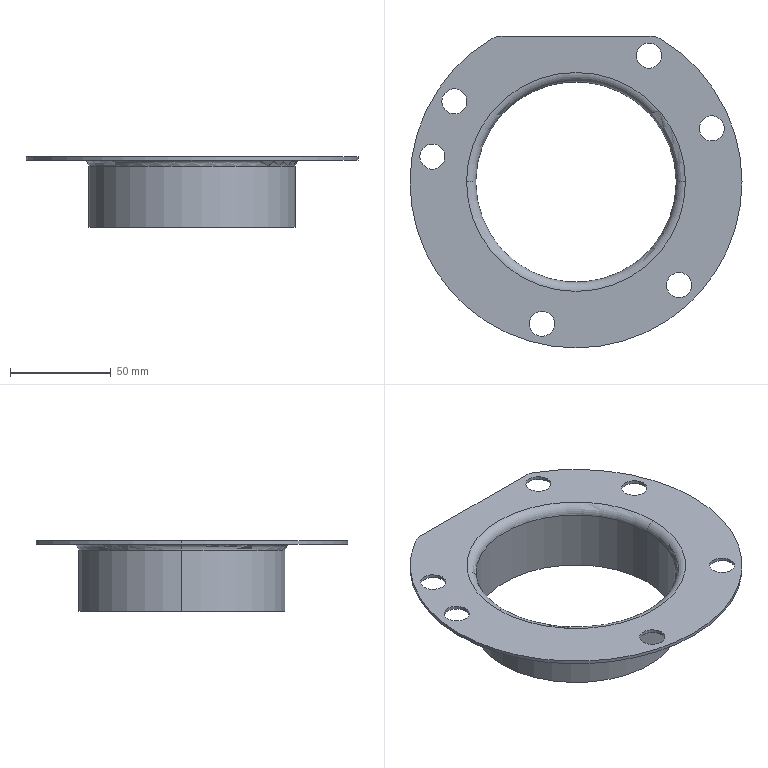Part | SolidWorks | features ICE 2, CirPattern 1, Fillet 1, RevolutionThin 1 | 1 solid | 29 faces | box 165 x 155 x 35 mm | volume 35887 mm3 | cylinder 21 | torus 4 | plane 4 | commonest cylinder face diameters 12.5 x12 165 x3 20 x2 99.6 x2 102.8 x2
STEP:
#1=CARTESIAN_POINT('',(30.,62.787,33.4));
#2=VERTEX_POINT('',#1);
#3=CARTESIAN_POINT('',(42.5,62.787,33.4));
#4=VERTEX_POINT('',#3);
#5=CARTESIAN_POINT('',(36.25,62.787,33.4));
#6=DIRECTION('',(0.,0.,1.));
#7=DIRECTION('',(-1.,0.,0.));
#8=AXIS2_PLACEMENT_3D('',#5,#6,#7);
#9=CIRCLE('',#8,6.25);
#10=EDGE_CURVE('',#2,#4,#9,.T.);
#11=ORIENTED_EDGE('',*,*,#10,.F.);
#12=CARTESIAN_POINT('',(30.,62.787,35.));
#13=VERTEX_POINT('',#12);
#14=CARTESIAN_POINT('',(30.,62.787,-0.001));
#15=DIRECTION('',(0.,0.,1.));
#16=VECTOR('',#15,1000.);
#17=LINE('',#14,#16);
#18=EDGE_CURVE('',#2,#13,#17,.T.);
#19=ORIENTED_EDGE('',*,*,#18,.T.);
#20=CARTESIAN_POINT('',(42.5,62.787,35.));
#21=VERTEX_POINT('',#20);
#22=CARTESIAN_POINT('',(36.25,62.787,35.));
#23=DIRECTION('',(0.,0.,1.));
#24=DIRECTION('',(1.,0.,0.));
#25=AXIS2_PLACEMENT_3D('',#22,#23,#24);
#26=CIRCLE('',#25,6.25);
#27=EDGE_CURVE('',#13,#21,#26,.T.);
#28=ORIENTED_EDGE('',*,*,#27,.T.);
#29=CARTESIAN_POINT('',(42.5,62.787,-0.001));
#30=DIRECTION('',(0.,0.,1.));
#31=VECTOR('',#30,1000.);
#32=LINE('',#29,#31);
#33=EDGE_CURVE('',#4,#21,#32,.T.);
#34=ORIENTED_EDGE('',*,*,#33,.F.);
#35=EDGE_LOOP('',(#11,#19,#28,#34));
#36=FACE_OUTER_BOUND('',#35,.T.);
#37=CARTESIAN_POINT('',(36.25,62.787,-0.001));
#38=DIRECTION('',(0.,0.,1.));
#39=DIRECTION('',(1.,0.,0.));
#40=AXIS2_PLACEMENT_3D('',#37,#38,#39);
#41=CYLINDRICAL_SURFACE('',#40,6.25);
#42=ADVANCED_FACE('',(#36),#41,.F.);
#43=CARTESIAN_POINT('',(61.205,26.571,33.4));
#44=VERTEX_POINT('',#43);
#45=CARTESIAN_POINT('',(73.705,26.571,33.4));
#46=VERTEX_POINT('',#45);
#47=CARTESIAN_POINT('',(67.455,26.571,33.4));
#48=DIRECTION('',(0.,0.,1.));
#49=DIRECTION('',(-1.,0.,0.));
#50=AXIS2_PLACEMENT_3D('',#47,#48,#49);
#51=CIRCLE('',#50,6.25);
#52=EDGE_CURVE('',#44,#46,#51,.T.);
#53=ORIENTED_EDGE('',*,*,#52,.F.);
#54=CARTESIAN_POINT('',(61.205,26.571,35.));
#55=VERTEX_POINT('',#54);
#56=CARTESIAN_POINT('',(61.205,26.571,-0.001));
#57=DIRECTION('',(0.,0.,1.));
#58=VECTOR('',#57,1000.);
#59=LINE('',#56,#58);
#60=EDGE_CURVE('',#44,#55,#59,.T.);
#61=ORIENTED_EDGE('',*,*,#60,.T.);
#62=CARTESIAN_POINT('',(73.705,26.571,35.));
#63=VERTEX_POINT('',#62);
#64=CARTESIAN_POINT('',(67.455,26.571,35.));
#65=DIRECTION('',(0.,0.,1.));
#66=DIRECTION('',(1.,0.,0.));
#67=AXIS2_PLACEMENT_3D('',#64,#65,#66);
#68=CIRCLE('',#67,6.25);
#69=EDGE_CURVE('',#55,#63,#68,.T.);
#70=ORIENTED_EDGE('',*,*,#69,.T.);
#71=CARTESIAN_POINT('',(73.705,26.571,-0.001));
#72=DIRECTION('',(0.,0.,1.));
#73=VECTOR('',#72,1000.);
#74=LINE('',#71,#73);
#75=EDGE_CURVE('',#46,#63,#74,.T.);
#76=ORIENTED_EDGE('',*,*,#75,.F.);
#77=EDGE_LOOP('',(#53,#61,#70,#76));
#78=FACE_OUTER_BOUND('',#77,.T.);
#79=CARTESIAN_POINT('',(67.455,26.571,-0.001));
#80=DIRECTION('',(0.,0.,1.));
#81=DIRECTION('',(1.,0.,0.));
#82=AXIS2_PLACEMENT_3D('',#79,#80,#81);
#83=CYLINDRICAL_SURFACE('',#82,6.25);
#84=ADVANCED_FACE('',(#78),#83,.F.);
#85=CARTESIAN_POINT('',(45.015,-51.265,33.4));
#86=VERTEX_POINT('',#85);
#87=CARTESIAN_POINT('',(57.515,-51.265,33.4));
#88=VERTEX_POINT('',#87);
#89=CARTESIAN_POINT('',(51.265,-51.265,33.4));
#90=DIRECTION('',(0.,0.,1.));
#91=DIRECTION('',(-1.,0.,0.));
#92=AXIS2_PLACEMENT_3D('',#89,#90,#91);
#93=CIRCLE('',#92,6.25);
#94=EDGE_CURVE('',#86,#88,#93,.T.);
#95=ORIENTED_EDGE('',*,*,#94,.F.);
#96=CARTESIAN_POINT('',(45.015,-51.265,35.));
#97=VERTEX_POINT('',#96);
#98=CARTESIAN_POINT('',(45.015,-51.265,-0.001));
#99=DIRECTION('',(0.,0.,1.));
#100=VECTOR('',#99,1000.);
#101=LINE('',#98,#100);
#102=EDGE_CURVE('',#86,#97,#101,.T.);
#103=ORIENTED_EDGE('',*,*,#102,.T.);
#104=CARTESIAN_POINT('',(57.515,-51.265,35.));
#105=VERTEX_POINT('',#104);
#106=CARTESIAN_POINT('',(51.265,-51.265,35.));
#107=DIRECTION('',(0.,0.,1.));
#108=DIRECTION('',(1.,0.,0.));
#109=AXIS2_PLACEMENT_3D('',#106,#107,#108);
#110=CIRCLE('',#109,6.25);
#111=EDGE_CURVE('',#97,#105,#110,.T.);
#112=ORIENTED_EDGE('',*,*,#111,.T.);
#113=CARTESIAN_POINT('',(57.515,-51.265,-0.001));
#114=DIRECTION('',(0.,0.,1.));
#115=VECTOR('',#114,1000.);
#116=LINE('',#113,#115);
#117=EDGE_CURVE('',#88,#105,#116,.T.);
#118=ORIENTED_EDGE('',*,*,#117,.F.);
#119=EDGE_LOOP('',(#95,#103,#112,#118));
#120=FACE_OUTER_BOUND('',#119,.T.);
#121=CARTESIAN_POINT('',(51.265,-51.265,-0.001));
#122=DIRECTION('',(0.,0.,1.));
#123=DIRECTION('',(1.,0.,0.));
#124=AXIS2_PLACEMENT_3D('',#121,#122,#123);
#125=CYLINDRICAL_SURFACE('',#124,6.25);
#126=ADVANCED_FACE('',(#120),#125,.F.);
#127=CARTESIAN_POINT('',(-23.175,-70.497,33.4));
#128=VERTEX_POINT('',#127);
#129=CARTESIAN_POINT('',(-10.675,-70.497,33.4));
#130=VERTEX_POINT('',#129);
#131=CARTESIAN_POINT('',(-16.925,-70.497,33.4));
#132=DIRECTION('',(0.,0.,1.));
#133=DIRECTION('',(-1.,0.,0.));
#134=AXIS2_PLACEMENT_3D('',#131,#132,#133);
#135=CIRCLE('',#134,6.25);
#136=EDGE_CURVE('',#128,#130,#135,.T.);
#137=ORIENTED_EDGE('',*,*,#136,.F.);
#138=CARTESIAN_POINT('',(-23.175,-70.497,35.));
#139=VERTEX_POINT('',#138);
#140=CARTESIAN_POINT('',(-23.175,-70.497,-0.001));
#141=DIRECTION('',(0.,0.,1.));
#142=VECTOR('',#141,1000.);
#143=LINE('',#140,#142);
#144=EDGE_CURVE('',#128,#139,#143,.T.);
#145=ORIENTED_EDGE('',*,*,#144,.T.);
#146=CARTESIAN_POINT('',(-10.675,-70.497,35.));
#147=VERTEX_POINT('',#146);
#148=CARTESIAN_POINT('',(-16.925,-70.497,35.));
#149=DIRECTION('',(0.,0.,1.));
#150=DIRECTION('',(1.,0.,0.));
#151=AXIS2_PLACEMENT_3D('',#148,#149,#150);
#152=CIRCLE('',#151,6.25);
#153=EDGE_CURVE('',#139,#147,#152,.T.);
#154=ORIENTED_EDGE('',*,*,#153,.T.);
#155=CARTESIAN_POINT('',(-10.675,-70.497,-0.001));
#156=DIRECTION('',(0.,0.,1.));
#157=VECTOR('',#156,1000.);
#158=LINE('',#155,#157);
#159=EDGE_CURVE('',#130,#147,#158,.T.);
#160=ORIENTED_EDGE('',*,*,#159,.F.);
#161=EDGE_LOOP('',(#137,#145,#154,#160));
#162=FACE_OUTER_BOUND('',#161,.T.);
#163=CARTESIAN_POINT('',(-16.925,-70.497,-0.001));
#164=DIRECTION('',(0.,0.,1.));
#165=DIRECTION('',(1.,0.,0.));
#166=AXIS2_PLACEMENT_3D('',#163,#164,#165);
#167=CYLINDRICAL_SURFACE('',#166,6.25);
#168=ADVANCED_FACE('',(#162),#167,.F.);
#169=CARTESIAN_POINT('',(-77.649,12.589,33.4));
#170=VERTEX_POINT('',#169);
#171=CARTESIAN_POINT('',(-65.149,12.589,33.4));
#172=VERTEX_POINT('',#171);
#173=CARTESIAN_POINT('',(-71.399,12.589,33.4));
#174=DIRECTION('',(0.,0.,1.));
#175=DIRECTION('',(-1.,0.,0.));
#176=AXIS2_PLACEMENT_3D('',#173,#174,#175);
#177=CIRCLE('',#176,6.25);
#178=EDGE_CURVE('',#170,#172,#177,.T.);
#179=ORIENTED_EDGE('',*,*,#178,.F.);
#180=CARTESIAN_POINT('',(-77.649,12.589,35.));
#181=VERTEX_POINT('',#180);
#182=CARTESIAN_POINT('',(-77.649,12.589,-0.001));
#183=DIRECTION('',(0.,0.,1.));
#184=VECTOR('',#183,1000.);
#185=LINE('',#182,#184);
#186=EDGE_CURVE('',#170,#181,#185,.T.);
#187=ORIENTED_EDGE('',*,*,#186,.T.);
#188=CARTESIAN_POINT('',(-65.149,12.589,35.));
#189=VERTEX_POINT('',#188);
#190=CARTESIAN_POINT('',(-71.399,12.589,35.));
#191=DIRECTION('',(0.,0.,1.));
#192=DIRECTION('',(1.,0.,0.));
#193=AXIS2_PLACEMENT_3D('',#190,#191,#192);
#194=CIRCLE('',#193,6.25);
#195=EDGE_CURVE('',#181,#189,#194,.T.);
#196=ORIENTED_EDGE('',*,*,#195,.T.);
#197=CARTESIAN_POINT('',(-65.149,12.589,-0.001));
#198=DIRECTION('',(0.,0.,1.));
#199=VECTOR('',#198,1000.);
#200=LINE('',#197,#199);
#201=EDGE_CURVE('',#172,#189,#200,.T.);
#202=ORIENTED_EDGE('',*,*,#201,.F.);
#203=EDGE_LOOP('',(#179,#187,#196,#202));
#204=FACE_OUTER_BOUND('',#203,.T.);
#205=CARTESIAN_POINT('',(-71.399,12.589,-0.001));
#206=DIRECTION('',(0.,0.,1.));
#207=DIRECTION('',(1.,0.,0.));
#208=AXIS2_PLACEMENT_3D('',#205,#206,#207);
#209=CYLINDRICAL_SURFACE('',#208,6.25);
#210=ADVANCED_FACE('',(#204),#209,.F.);
#211=CARTESIAN_POINT('',(-66.707,40.015,33.4));
#212=VERTEX_POINT('',#211);
#213=CARTESIAN_POINT('',(-54.207,40.015,33.4));
#214=VERTEX_POINT('',#213);
#215=CARTESIAN_POINT('',(-60.457,40.015,33.4));
#216=DIRECTION('',(0.,0.,1.));
#217=DIRECTION('',(-1.,0.,0.));
#218=AXIS2_PLACEMENT_3D('',#215,#216,#217);
#219=CIRCLE('',#218,6.25);
#220=EDGE_CURVE('',#212,#214,#219,.T.);
#221=ORIENTED_EDGE('',*,*,#220,.F.);
#222=CARTESIAN_POINT('',(-66.707,40.015,35.));
#223=VERTEX_POINT('',#222);
#224=CARTESIAN_POINT('',(-66.707,40.015,-0.001));
#225=DIRECTION('',(0.,0.,1.));
#226=VECTOR('',#225,1000.);
#227=LINE('',#224,#226);
#228=EDGE_CURVE('',#212,#223,#227,.T.);
#229=ORIENTED_EDGE('',*,*,#228,.T.);
#230=CARTESIAN_POINT('',(-54.207,40.015,35.));
#231=VERTEX_POINT('',#230);
#232=CARTESIAN_POINT('',(-60.457,40.015,35.));
#233=DIRECTION('',(0.,0.,1.));
#234=DIRECTION('',(1.,0.,0.));
#235=AXIS2_PLACEMENT_3D('',#232,#233,#234);
#236=CIRCLE('',#235,6.25);
#237=EDGE_CURVE('',#223,#231,#236,.T.);
#238=ORIENTED_EDGE('',*,*,#237,.T.);
#239=CARTESIAN_POINT('',(-54.207,40.015,-0.001));
#240=DIRECTION('',(0.,0.,1.));
#241=VECTOR('',#240,1000.);
#242=LINE('',#239,#241);
#243=EDGE_CURVE('',#214,#231,#242,.T.);
#244=ORIENTED_EDGE('',*,*,#243,.F.);
#245=EDGE_LOOP('',(#221,#229,#238,#244));
#246=FACE_OUTER_BOUND('',#245,.T.);
#247=CARTESIAN_POINT('',(-60.457,40.015,-0.001));
#248=DIRECTION('',(0.,0.,1.));
#249=DIRECTION('',(1.,0.,0.));
#250=AXIS2_PLACEMENT_3D('',#247,#248,#249);
#251=CYLINDRICAL_SURFACE('',#250,6.25);
#252=ADVANCED_FACE('',(#246),#251,.F.);
#253=CARTESIAN_POINT('',(41.81,71.121,35.));
#254=VERTEX_POINT('',#253);
#255=CARTESIAN_POINT('',(82.5,0.,35.));
#256=VERTEX_POINT('',#255);
#257=CARTESIAN_POINT('',(0.,0.,35.));
#258=DIRECTION('',(0.,0.,-1.));
#259=DIRECTION('',(-1.,0.,0.));
#260=AXIS2_PLACEMENT_3D('',#257,#258,#259);
#261=CIRCLE('',#260,82.5);
#262=EDGE_CURVE('',#254,#256,#261,.T.);
#263=ORIENTED_EDGE('',*,*,#262,.T.);
#264=CARTESIAN_POINT('',(82.5,0.,33.4));
#265=VERTEX_POINT('',#264);
#266=CARTESIAN_POINT('',(82.5,0.,0.));
#267=DIRECTION('',(0.,0.,-1.));
#268=VECTOR('',#267,1000.);
#269=LINE('',#266,#268);
#270=EDGE_CURVE('',#256,#265,#269,.T.);
#271=ORIENTED_EDGE('',*,*,#270,.T.);
#272=CARTESIAN_POINT('',(41.81,71.121,33.4));
#273=VERTEX_POINT('',#272);
#274=CARTESIAN_POINT('',(0.,0.,33.4));
#275=DIRECTION('',(0.,0.,-1.));
#276=DIRECTION('',(-1.,0.,0.));
#277=AXIS2_PLACEMENT_3D('',#274,#275,#276);
#278=CIRCLE('',#277,82.5);
#279=EDGE_CURVE('',#273,#265,#278,.T.);
#280=ORIENTED_EDGE('',*,*,#279,.F.);
#281=CARTESIAN_POINT('',(41.81,71.121,0.));
#282=DIRECTION('',(0.,0.,1.));
#283=VECTOR('',#282,1000.);
#284=LINE('',#281,#283);
#285=EDGE_CURVE('',#273,#254,#284,.T.);
#286=ORIENTED_EDGE('',*,*,#285,.T.);
#287=EDGE_LOOP('',(#263,#271,#280,#286));
#288=FACE_OUTER_BOUND('',#287,.T.);
#289=CARTESIAN_POINT('',(0.,0.,0.));
#290=DIRECTION('',(0.,0.,-1.));
#291=DIRECTION('',(-1.,0.,0.));
#292=AXIS2_PLACEMENT_3D('',#289,#290,#291);
#293=CYLINDRICAL_SURFACE('',#292,82.5);
#294=ADVANCED_FACE('',(#288),#293,.T.);
#295=ORIENTED_EDGE('',*,*,#270,.F.);
#296=CARTESIAN_POINT('',(-82.5,0.,35.));
#297=VERTEX_POINT('',#296);
#298=CARTESIAN_POINT('',(0.,0.,35.));
#299=DIRECTION('',(0.,0.,-1.));
#300=DIRECTION('',(-1.,0.,0.));
#301=AXIS2_PLACEMENT_3D('',#298,#299,#300);
#302=CIRCLE('',#301,82.5);
#303=EDGE_CURVE('',#256,#297,#302,.T.);
#304=ORIENTED_EDGE('',*,*,#303,.T.);
#305=CARTESIAN_POINT('',(-82.5,0.,33.4));
#306=VERTEX_POINT('',#305);
#307=CARTESIAN_POINT('',(-82.5,0.,0.));
#308=DIRECTION('',(0.,0.,-1.));
#309=VECTOR('',#308,1000.);
#310=LINE('',#307,#309);
#311=EDGE_CURVE('',#297,#306,#310,.T.);
#312=ORIENTED_EDGE('',*,*,#311,.T.);
#313=CARTESIAN_POINT('',(0.,0.,33.4));
#314=DIRECTION('',(0.,0.,-1.));
#315=DIRECTION('',(-1.,0.,0.));
#316=AXIS2_PLACEMENT_3D('',#313,#314,#315);
#317=CIRCLE('',#316,82.5);
#318=EDGE_CURVE('',#265,#306,#317,.T.);
#319=ORIENTED_EDGE('',*,*,#318,.F.);
#320=EDGE_LOOP('',(#295,#304,#312,#319));
#321=FACE_OUTER_BOUND('',#320,.T.);
#322=CARTESIAN_POINT('',(0.,0.,0.));
#323=DIRECTION('',(0.,0.,-1.));
#324=DIRECTION('',(-1.,0.,0.));
#325=AXIS2_PLACEMENT_3D('',#322,#323,#324);
#326=CYLINDRICAL_SURFACE('',#325,82.5);
#327=ADVANCED_FACE('',(#321),#326,.T.);
#328=CARTESIAN_POINT('',(-49.8,0.,30.4));
#329=VERTEX_POINT('',#328);
#330=CARTESIAN_POINT('',(49.8,0.,30.4));
#331=VERTEX_POINT('',#330);
#332=CARTESIAN_POINT('',(0.,0.,30.4));
#333=DIRECTION('',(0.,0.,-1.));
#334=DIRECTION('',(-1.,0.,0.));
#335=AXIS2_PLACEMENT_3D('',#332,#333,#334);
#336=CIRCLE('',#335,49.8);
#337=EDGE_CURVE('',#329,#331,#336,.T.);
#338=ORIENTED_EDGE('',*,*,#337,.T.);
#339=CARTESIAN_POINT('',(54.4,0.,35.));
#340=VERTEX_POINT('',#339);
#341=CARTESIAN_POINT('',(54.4,0.,30.4));
#342=DIRECTION('',(0.,1.,0.));
#343=DIRECTION('',(-1.,0.,0.));
#344=AXIS2_PLACEMENT_3D('',#341,#342,#343);
#345=CIRCLE('',#344,4.6);
#346=EDGE_CURVE('',#331,#340,#345,.T.);
#347=ORIENTED_EDGE('',*,*,#346,.T.);
#348=CARTESIAN_POINT('',(-54.4,0.,35.));
#349=VERTEX_POINT('',#348);
#350=CARTESIAN_POINT('',(0.,0.,35.));
#351=DIRECTION('',(0.,0.,-1.));
#352=DIRECTION('',(-1.,0.,0.));
#353=AXIS2_PLACEMENT_3D('',#350,#351,#352);
#354=CIRCLE('',#353,54.4);
#355=EDGE_CURVE('',#349,#340,#354,.T.);
#356=ORIENTED_EDGE('',*,*,#355,.F.);
#357=CARTESIAN_POINT('',(-54.4,0.,30.4));
#358=DIRECTION('',(0.,-1.,0.));
#359=DIRECTION('',(0.,0.,-1.));
#360=AXIS2_PLACEMENT_3D('',#357,#358,#359);
#361=CIRCLE('',#360,4.6);
#362=EDGE_CURVE('',#329,#349,#361,.T.);
#363=ORIENTED_EDGE('',*,*,#362,.F.);
#364=EDGE_LOOP('',(#338,#347,#356,#363));
#365=FACE_OUTER_BOUND('',#364,.T.);
#366=CARTESIAN_POINT('',(0.,0.,30.4));
#367=DIRECTION('',(0.,0.,-1.));
#368=DIRECTION('',(-1.,0.,0.));
#369=AXIS2_PLACEMENT_3D('',#366,#367,#368);
#370=TOROIDAL_SURFACE('',#369,54.4,4.6);
#371=ADVANCED_FACE('',(#365),#370,.T.);
#372=CARTESIAN_POINT('',(0.,0.,30.4));
#373=DIRECTION('',(0.,0.,-1.));
#374=DIRECTION('',(-1.,0.,0.));
#375=AXIS2_PLACEMENT_3D('',#372,#373,#374);
#376=CIRCLE('',#375,49.8);
#377=EDGE_CURVE('',#331,#329,#376,.T.);
#378=ORIENTED_EDGE('',*,*,#377,.F.);
#379=CARTESIAN_POINT('',(49.8,0.,0.));
#380=VERTEX_POINT('',#379);
#381=CARTESIAN_POINT('',(49.8,0.,0.));
#382=DIRECTION('',(0.,0.,-1.));
#383=VECTOR('',#382,1000.);
#384=LINE('',#381,#383);
#385=EDGE_CURVE('',#331,#380,#384,.T.);
#386=ORIENTED_EDGE('',*,*,#385,.T.);
#387=CARTESIAN_POINT('',(-49.8,0.,0.));
#388=VERTEX_POINT('',#387);
#389=CARTESIAN_POINT('',(0.,0.,0.));
#390=DIRECTION('',(0.,0.,-1.));
#391=DIRECTION('',(-1.,0.,0.));
#392=AXIS2_PLACEMENT_3D('',#389,#390,#391);
#393=CIRCLE('',#392,49.8);
#394=EDGE_CURVE('',#380,#388,#393,.T.);
#395=ORIENTED_EDGE('',*,*,#394,.T.);
#396=CARTESIAN_POINT('',(-49.8,0.,0.));
#397=DIRECTION('',(0.,0.,-1.));
#398=VECTOR('',#397,1000.);
#399=LINE('',#396,#398);
#400=EDGE_CURVE('',#329,#388,#399,.T.);
#401=ORIENTED_EDGE('',*,*,#400,.F.);
#402=EDGE_LOOP('',(#378,#386,#395,#401));
#403=FACE_OUTER_BOUND('',#402,.T.);
#404=CARTESIAN_POINT('',(0.,0.,0.));
#405=DIRECTION('',(0.,0.,-1.));
#406=DIRECTION('',(-1.,0.,0.));
#407=AXIS2_PLACEMENT_3D('',#404,#405,#406);
#408=CYLINDRICAL_SURFACE('',#407,49.8);
#409=ADVANCED_FACE('',(#403),#408,.F.);
#410=CARTESIAN_POINT('',(-51.4,0.,30.4));
#411=VERTEX_POINT('',#410);
#412=CARTESIAN_POINT('',(51.4,0.,30.4));
#413=VERTEX_POINT('',#412);
#414=CARTESIAN_POINT('',(0.,0.,30.4));
#415=DIRECTION('',(0.,0.,-1.));
#416=DIRECTION('',(-1.,0.,0.));
#417=AXIS2_PLACEMENT_3D('',#414,#415,#416);
#418=CIRCLE('',#417,51.4);
#419=EDGE_CURVE('',#411,#413,#418,.T.);
#420=ORIENTED_EDGE('',*,*,#419,.T.);
#421=CARTESIAN_POINT('',(51.4,0.,0.));
#422=VERTEX_POINT('',#421);
#423=CARTESIAN_POINT('',(51.4,0.,0.));
#424=DIRECTION('',(0.,0.,-1.));
#425=VECTOR('',#424,1000.);
#426=LINE('',#423,#425);
#427=EDGE_CURVE('',#413,#422,#426,.T.);
#428=ORIENTED_EDGE('',*,*,#427,.T.);
#429=CARTESIAN_POINT('',(-51.4,0.,0.));
#430=VERTEX_POINT('',#429);
#431=CARTESIAN_POINT('',(0.,0.,0.));
#432=DIRECTION('',(0.,0.,-1.));
#433=DIRECTION('',(-1.,0.,0.));
#434=AXIS2_PLACEMENT_3D('',#431,#432,#433);
#435=CIRCLE('',#434,51.4);
#436=EDGE_CURVE('',#430,#422,#435,.T.);
#437=ORIENTED_EDGE('',*,*,#436,.F.);
#438=CARTESIAN_POINT('',(-51.4,0.,0.));
#439=DIRECTION('',(0.,0.,-1.));
#440=VECTOR('',#439,1000.);
#441=LINE('',#438,#440);
#442=EDGE_CURVE('',#411,#430,#441,.T.);
#443=ORIENTED_EDGE('',*,*,#442,.F.);
#444=EDGE_LOOP('',(#420,#428,#437,#443));
#445=FACE_OUTER_BOUND('',#444,.T.);
#446=CARTESIAN_POINT('',(0.,0.,0.));
#447=DIRECTION('',(0.,0.,-1.));
#448=DIRECTION('',(-1.,0.,0.));
#449=AXIS2_PLACEMENT_3D('',#446,#447,#448);
#450=CYLINDRICAL_SURFACE('',#449,51.4);
#451=ADVANCED_FACE('',(#445),#450,.T.);
#452=CARTESIAN_POINT('',(0.,0.,30.4));
#453=DIRECTION('',(0.,0.,-1.));
#454=DIRECTION('',(-1.,0.,0.));
#455=AXIS2_PLACEMENT_3D('',#452,#453,#454);
#456=CIRCLE('',#455,51.4);
#457=EDGE_CURVE('',#413,#411,#456,.T.);
#458=ORIENTED_EDGE('',*,*,#457,.F.);
#459=CARTESIAN_POINT('',(54.4,0.,33.4));
#460=VERTEX_POINT('',#459);
#461=CARTESIAN_POINT('',(54.4,0.,30.4));
#462=DIRECTION('',(0.,1.,0.));
#463=DIRECTION('',(-1.,0.,0.));
#464=AXIS2_PLACEMENT_3D('',#461,#462,#463);
#465=CIRCLE('',#464,3.);
#466=EDGE_CURVE('',#413,#460,#465,.T.);
#467=ORIENTED_EDGE('',*,*,#466,.T.);
#468=CARTESIAN_POINT('',(-54.4,0.,33.4));
#469=VERTEX_POINT('',#468);
#470=CARTESIAN_POINT('',(0.,0.,33.4));
#471=DIRECTION('',(0.,0.,-1.));
#472=DIRECTION('',(-1.,0.,0.));
#473=AXIS2_PLACEMENT_3D('',#470,#471,#472);
#474=CIRCLE('',#473,54.4);
#475=EDGE_CURVE('',#460,#469,#474,.T.);
#476=ORIENTED_EDGE('',*,*,#475,.T.);
#477=CARTESIAN_POINT('',(-54.4,0.,30.4));
#478=DIRECTION('',(0.,-1.,0.));
#479=DIRECTION('',(0.,0.,-1.));
#480=AXIS2_PLACEMENT_3D('',#477,#478,#479);
#481=CIRCLE('',#480,3.);
#482=EDGE_CURVE('',#411,#469,#481,.T.);
#483=ORIENTED_EDGE('',*,*,#482,.F.);
#484=EDGE_LOOP('',(#458,#467,#476,#483));
#485=FACE_OUTER_BOUND('',#484,.T.);
#486=CARTESIAN_POINT('',(0.,0.,30.4));
#487=DIRECTION('',(0.,0.,-1.));
#488=DIRECTION('',(-1.,0.,0.));
#489=AXIS2_PLACEMENT_3D('',#486,#487,#488);
#490=TOROIDAL_SURFACE('',#489,54.4,3.);
#491=ADVANCED_FACE('',(#485),#490,.F.);
#492=CARTESIAN_POINT('',(36.25,62.787,33.4));
#493=DIRECTION('',(0.,0.,1.));
#494=DIRECTION('',(-1.,0.,0.));
#495=AXIS2_PLACEMENT_3D('',#492,#493,#494);
#496=CIRCLE('',#495,6.25);
#497=EDGE_CURVE('',#4,#2,#496,.T.);
#498=ORIENTED_EDGE('',*,*,#497,.T.);
#499=ORIENTED_EDGE('',*,*,#10,.T.);
#500=EDGE_LOOP('',(#498,#499));
#501=FACE_BOUND('',#500,.T.);
#502=CARTESIAN_POINT('',(67.455,26.571,33.4));
#503=DIRECTION('',(0.,0.,1.));
#504=DIRECTION('',(-1.,0.,0.));
#505=AXIS2_PLACEMENT_3D('',#502,#503,#504);
#506=CIRCLE('',#505,6.25);
#507=EDGE_CURVE('',#46,#44,#506,.T.);
#508=ORIENTED_EDGE('',*,*,#507,.T.);
#509=ORIENTED_EDGE('',*,*,#52,.T.);
#510=EDGE_LOOP('',(#508,#509));
#511=FACE_BOUND('',#510,.T.);
#512=CARTESIAN_POINT('',(51.265,-51.265,33.4));
#513=DIRECTION('',(0.,0.,1.));
#514=DIRECTION('',(-1.,0.,0.));
#515=AXIS2_PLACEMENT_3D('',#512,#513,#514);
#516=CIRCLE('',#515,6.25);
#517=EDGE_CURVE('',#88,#86,#516,.T.);
#518=ORIENTED_EDGE('',*,*,#517,.T.);
#519=ORIENTED_EDGE('',*,*,#94,.T.);
#520=EDGE_LOOP('',(#518,#519));
#521=FACE_BOUND('',#520,.T.);
#522=CARTESIAN_POINT('',(-16.925,-70.497,33.4));
#523=DIRECTION('',(0.,0.,1.));
#524=DIRECTION('',(-1.,0.,0.));
#525=AXIS2_PLACEMENT_3D('',#522,#523,#524);
#526=CIRCLE('',#525,6.25);
#527=EDGE_CURVE('',#130,#128,#526,.T.);
#528=ORIENTED_EDGE('',*,*,#527,.T.);
#529=ORIENTED_EDGE('',*,*,#136,.T.);
#530=EDGE_LOOP('',(#528,#529));
#531=FACE_BOUND('',#530,.T.);
#532=CARTESIAN_POINT('',(-71.399,12.589,33.4));
#533=DIRECTION('',(0.,0.,1.));
#534=DIRECTION('',(-1.,0.,0.));
#535=AXIS2_PLACEMENT_3D('',#532,#533,#534);
#536=CIRCLE('',#535,6.25);
#537=EDGE_CURVE('',#172,#170,#536,.T.);
#538=ORIENTED_EDGE('',*,*,#537,.T.);
#539=ORIENTED_EDGE('',*,*,#178,.T.);
#540=EDGE_LOOP('',(#538,#539));
#541=FACE_BOUND('',#540,.T.);
#542=CARTESIAN_POINT('',(-36.742,72.5,33.4));
#543=VERTEX_POINT('',#542);
#544=CARTESIAN_POINT('',(36.742,72.5,33.4));
#545=VERTEX_POINT('',#544);
#546=CARTESIAN_POINT('',(-45.,72.5,33.4));
#547=DIRECTION('',(1.,0.,0.));
#548=VECTOR('',#547,1000.);
#549=LINE('',#546,#548);
#550=EDGE_CURVE('',#543,#545,#549,.T.);
#551=ORIENTED_EDGE('',*,*,#550,.T.);
#552=CARTESIAN_POINT('',(36.742,62.5,33.4));
#553=DIRECTION('',(0.,0.,-1.));
#554=DIRECTION('',(-1.,0.,0.));
#555=AXIS2_PLACEMENT_3D('',#552,#553,#554);
#556=CIRCLE('',#555,10.);
#557=EDGE_CURVE('',#545,#273,#556,.T.);
#558=ORIENTED_EDGE('',*,*,#557,.T.);
#559=ORIENTED_EDGE('',*,*,#279,.T.);
#560=ORIENTED_EDGE('',*,*,#318,.T.);
#561=CARTESIAN_POINT('',(-41.81,71.121,33.4));
#562=VERTEX_POINT('',#561);
#563=CARTESIAN_POINT('',(0.,0.,33.4));
#564=DIRECTION('',(0.,0.,-1.));
#565=DIRECTION('',(-1.,0.,0.));
#566=AXIS2_PLACEMENT_3D('',#563,#564,#565);
#567=CIRCLE('',#566,82.5);
#568=EDGE_CURVE('',#306,#562,#567,.T.);
#569=ORIENTED_EDGE('',*,*,#568,.T.);
#570=CARTESIAN_POINT('',(-36.742,62.5,33.4));
#571=DIRECTION('',(0.,0.,-1.));
#572=DIRECTION('',(-1.,0.,0.));
#573=AXIS2_PLACEMENT_3D('',#570,#571,#572);
#574=CIRCLE('',#573,10.);
#575=EDGE_CURVE('',#562,#543,#574,.T.);
#576=ORIENTED_EDGE('',*,*,#575,.T.);
#577=EDGE_LOOP('',(#551,#558,#559,#560,#569,#576));
#578=FACE_OUTER_BOUND('',#577,.T.);
#579=CARTESIAN_POINT('',(-60.457,40.015,33.4));
#580=DIRECTION('',(0.,0.,1.));
#581=DIRECTION('',(-1.,0.,0.));
#582=AXIS2_PLACEMENT_3D('',#579,#580,#581);
#583=CIRCLE('',#582,6.25);
#584=EDGE_CURVE('',#214,#212,#583,.T.);
#585=ORIENTED_EDGE('',*,*,#584,.T.);
#586=ORIENTED_EDGE('',*,*,#220,.T.);
#587=EDGE_LOOP('',(#585,#586));
#588=FACE_BOUND('',#587,.T.);
#589=CARTESIAN_POINT('',(0.,0.,33.4));
#590=DIRECTION('',(0.,0.,-1.));
#591=DIRECTION('',(-1.,0.,0.));
#592=AXIS2_PLACEMENT_3D('',#589,#590,#591);
#593=CIRCLE('',#592,54.4);
#594=EDGE_CURVE('',#469,#460,#593,.T.);
#595=ORIENTED_EDGE('',*,*,#594,.F.);
#596=ORIENTED_EDGE('',*,*,#475,.F.);
#597=EDGE_LOOP('',(#595,#596));
#598=FACE_BOUND('',#597,.T.);
#599=CARTESIAN_POINT('',(0.,54.4,33.4));
#600=DIRECTION('',(0.,0.,-1.));
#601=DIRECTION('',(-1.,0.,0.));
#602=AXIS2_PLACEMENT_3D('',#599,#600,#601);
#603=PLANE('',#602);
#604=ADVANCED_FACE('',(#501,#511,#521,#531,#541,#578,#588,#598),#603,.T.);
#605=ORIENTED_EDGE('',*,*,#466,.F.);
#606=ORIENTED_EDGE('',*,*,#419,.F.);
#607=ORIENTED_EDGE('',*,*,#482,.T.);
#608=ORIENTED_EDGE('',*,*,#594,.T.);
#609=EDGE_LOOP('',(#605,#606,#607,#608));
#610=FACE_OUTER_BOUND('',#609,.T.);
#611=CARTESIAN_POINT('',(0.,0.,30.4));
#612=DIRECTION('',(0.,0.,-1.));
#613=DIRECTION('',(-1.,0.,0.));
#614=AXIS2_PLACEMENT_3D('',#611,#612,#613);
#615=TOROIDAL_SURFACE('',#614,54.4,3.);
#616=ADVANCED_FACE('',(#610),#615,.F.);
#617=ORIENTED_EDGE('',*,*,#427,.F.);
#618=ORIENTED_EDGE('',*,*,#457,.T.);
#619=ORIENTED_EDGE('',*,*,#442,.T.);
#620=CARTESIAN_POINT('',(0.,0.,0.));
#621=DIRECTION('',(0.,0.,-1.));
#622=DIRECTION('',(-1.,0.,0.));
#623=AXIS2_PLACEMENT_3D('',#620,#621,#622);
#624=CIRCLE('',#623,51.4);
#625=EDGE_CURVE('',#422,#430,#624,.T.);
#626=ORIENTED_EDGE('',*,*,#625,.F.);
#627=EDGE_LOOP('',(#617,#618,#619,#626));
#628=FACE_OUTER_BOUND('',#627,.T.);
#629=CARTESIAN_POINT('',(0.,0.,0.));
#630=DIRECTION('',(0.,0.,-1.));
#631=DIRECTION('',(-1.,0.,0.));
#632=AXIS2_PLACEMENT_3D('',#629,#630,#631);
#633=CYLINDRICAL_SURFACE('',#632,51.4);
#634=ADVANCED_FACE('',(#628),#633,.T.);
#635=CARTESIAN_POINT('',(0.,0.,0.));
#636=DIRECTION('',(0.,0.,-1.));
#637=DIRECTION('',(-1.,0.,0.));
#638=AXIS2_PLACEMENT_3D('',#635,#636,#637);
#639=CIRCLE('',#638,49.8);
#640=EDGE_CURVE('',#388,#380,#639,.T.);
#641=ORIENTED_EDGE('',*,*,#640,.F.);
#642=ORIENTED_EDGE('',*,*,#394,.F.);
#643=EDGE_LOOP('',(#641,#642));
#644=FACE_BOUND('',#643,.T.);
#645=ORIENTED_EDGE('',*,*,#436,.T.);
#646=ORIENTED_EDGE('',*,*,#625,.T.);
#647=EDGE_LOOP('',(#645,#646));
#648=FACE_OUTER_BOUND('',#647,.T.);
#649=CARTESIAN_POINT('',(0.,51.4,0.));
#650=DIRECTION('',(0.,0.,1.));
#651=DIRECTION('',(1.,0.,0.));
#652=AXIS2_PLACEMENT_3D('',#649,#650,#651);
#653=PLANE('',#652);
#654=ADVANCED_FACE('',(#644,#648),#653,.F.);
#655=ORIENTED_EDGE('',*,*,#385,.F.);
#656=ORIENTED_EDGE('',*,*,#337,.F.);
#657=ORIENTED_EDGE('',*,*,#400,.T.);
#658=ORIENTED_EDGE('',*,*,#640,.T.);
#659=EDGE_LOOP('',(#655,#656,#657,#658));
#660=FACE_OUTER_BOUND('',#659,.T.);
#661=CARTESIAN_POINT('',(0.,0.,0.));
#662=DIRECTION('',(0.,0.,-1.));
#663=DIRECTION('',(-1.,0.,0.));
#664=AXIS2_PLACEMENT_3D('',#661,#662,#663);
#665=CYLINDRICAL_SURFACE('',#664,49.8);
#666=ADVANCED_FACE('',(#660),#665,.F.);
#667=ORIENTED_EDGE('',*,*,#346,.F.);
#668=ORIENTED_EDGE('',*,*,#377,.T.);
#669=ORIENTED_EDGE('',*,*,#362,.T.);
#670=CARTESIAN_POINT('',(0.,0.,35.));
#671=DIRECTION('',(0.,0.,-1.));
#672=DIRECTION('',(-1.,0.,0.));
#673=AXIS2_PLACEMENT_3D('',#670,#671,#672);
#674=CIRCLE('',#673,54.4);
#675=EDGE_CURVE('',#340,#349,#674,.T.);
#676=ORIENTED_EDGE('',*,*,#675,.F.);
#677=EDGE_LOOP('',(#667,#668,#669,#676));
#678=FACE_OUTER_BOUND('',#677,.T.);
#679=CARTESIAN_POINT('',(0.,0.,30.4));
#680=DIRECTION('',(0.,0.,-1.));
#681=DIRECTION('',(-1.,0.,0.));
#682=AXIS2_PLACEMENT_3D('',#679,#680,#681);
#683=TOROIDAL_SURFACE('',#682,54.4,4.6);
#684=ADVANCED_FACE('',(#678),#683,.T.);
#685=CARTESIAN_POINT('',(36.25,62.787,35.));
#686=DIRECTION('',(0.,0.,1.));
#687=DIRECTION('',(1.,0.,0.));
#688=AXIS2_PLACEMENT_3D('',#685,#686,#687);
#689=CIRCLE('',#688,6.25);
#690=EDGE_CURVE('',#21,#13,#689,.T.);
#691=ORIENTED_EDGE('',*,*,#690,.F.);
#692=ORIENTED_EDGE('',*,*,#27,.F.);
#693=EDGE_LOOP('',(#691,#692));
#694=FACE_BOUND('',#693,.T.);
#695=CARTESIAN_POINT('',(67.455,26.571,35.));
#696=DIRECTION('',(0.,0.,1.));
#697=DIRECTION('',(1.,0.,0.));
#698=AXIS2_PLACEMENT_3D('',#695,#696,#697);
#699=CIRCLE('',#698,6.25);
#700=EDGE_CURVE('',#63,#55,#699,.T.);
#701=ORIENTED_EDGE('',*,*,#700,.F.);
#702=ORIENTED_EDGE('',*,*,#69,.F.);
#703=EDGE_LOOP('',(#701,#702));
#704=FACE_BOUND('',#703,.T.);
#705=CARTESIAN_POINT('',(51.265,-51.265,35.));
#706=DIRECTION('',(0.,0.,1.));
#707=DIRECTION('',(1.,0.,0.));
#708=AXIS2_PLACEMENT_3D('',#705,#706,#707);
#709=CIRCLE('',#708,6.25);
#710=EDGE_CURVE('',#105,#97,#709,.T.);
#711=ORIENTED_EDGE('',*,*,#710,.F.);
#712=ORIENTED_EDGE('',*,*,#111,.F.);
#713=EDGE_LOOP('',(#711,#712));
#714=FACE_BOUND('',#713,.T.);
#715=CARTESIAN_POINT('',(-16.925,-70.497,35.));
#716=DIRECTION('',(0.,0.,1.));
#717=DIRECTION('',(1.,0.,0.));
#718=AXIS2_PLACEMENT_3D('',#715,#716,#717);
#719=CIRCLE('',#718,6.25);
#720=EDGE_CURVE('',#147,#139,#719,.T.);
#721=ORIENTED_EDGE('',*,*,#720,.F.);
#722=ORIENTED_EDGE('',*,*,#153,.F.);
#723=EDGE_LOOP('',(#721,#722));
#724=FACE_BOUND('',#723,.T.);
#725=CARTESIAN_POINT('',(-71.399,12.589,35.));
#726=DIRECTION('',(0.,0.,1.));
#727=DIRECTION('',(1.,0.,0.));
#728=AXIS2_PLACEMENT_3D('',#725,#726,#727);
#729=CIRCLE('',#728,6.25);
#730=EDGE_CURVE('',#189,#181,#729,.T.);
#731=ORIENTED_EDGE('',*,*,#730,.F.);
#732=ORIENTED_EDGE('',*,*,#195,.F.);
#733=EDGE_LOOP('',(#731,#732));
#734=FACE_BOUND('',#733,.T.);
#735=CARTESIAN_POINT('',(-60.457,40.015,35.));
#736=DIRECTION('',(0.,0.,1.));
#737=DIRECTION('',(1.,0.,0.));
#738=AXIS2_PLACEMENT_3D('',#735,#736,#737);
#739=CIRCLE('',#738,6.25);
#740=EDGE_CURVE('',#231,#223,#739,.T.);
#741=ORIENTED_EDGE('',*,*,#740,.F.);
#742=ORIENTED_EDGE('',*,*,#237,.F.);
#743=EDGE_LOOP('',(#741,#742));
#744=FACE_BOUND('',#743,.T.);
#745=ORIENTED_EDGE('',*,*,#262,.F.);
#746=CARTESIAN_POINT('',(36.742,72.5,35.));
#747=VERTEX_POINT('',#746);
#748=CARTESIAN_POINT('',(36.742,62.5,35.));
#749=DIRECTION('',(0.,0.,1.));
#750=DIRECTION('',(-1.,0.,0.));
#751=AXIS2_PLACEMENT_3D('',#748,#749,#750);
#752=CIRCLE('',#751,10.);
#753=EDGE_CURVE('',#254,#747,#752,.T.);
#754=ORIENTED_EDGE('',*,*,#753,.T.);
#755=CARTESIAN_POINT('',(-36.742,72.5,35.));
#756=VERTEX_POINT('',#755);
#757=CARTESIAN_POINT('',(-45.,72.5,35.));
#758=DIRECTION('',(1.,0.,0.));
#759=VECTOR('',#758,1000.);
#760=LINE('',#757,#759);
#761=EDGE_CURVE('',#756,#747,#760,.T.);
#762=ORIENTED_EDGE('',*,*,#761,.F.);
#763=CARTESIAN_POINT('',(-41.81,71.121,35.));
#764=VERTEX_POINT('',#763);
#765=CARTESIAN_POINT('',(-36.742,62.5,35.));
#766=DIRECTION('',(0.,0.,1.));
#767=DIRECTION('',(-1.,0.,0.));
#768=AXIS2_PLACEMENT_3D('',#765,#766,#767);
#769=CIRCLE('',#768,10.);
#770=EDGE_CURVE('',#756,#764,#769,.T.);
#771=ORIENTED_EDGE('',*,*,#770,.T.);
#772=CARTESIAN_POINT('',(0.,0.,35.));
#773=DIRECTION('',(0.,0.,-1.));
#774=DIRECTION('',(-1.,0.,0.));
#775=AXIS2_PLACEMENT_3D('',#772,#773,#774);
#776=CIRCLE('',#775,82.5);
#777=EDGE_CURVE('',#297,#764,#776,.T.);
#778=ORIENTED_EDGE('',*,*,#777,.F.);
#779=ORIENTED_EDGE('',*,*,#303,.F.);
#780=EDGE_LOOP('',(#745,#754,#762,#771,#778,#779));
#781=FACE_OUTER_BOUND('',#780,.T.);
#782=ORIENTED_EDGE('',*,*,#355,.T.);
#783=ORIENTED_EDGE('',*,*,#675,.T.);
#784=EDGE_LOOP('',(#782,#783));
#785=FACE_BOUND('',#784,.T.);
#786=CARTESIAN_POINT('',(0.,54.4,35.));
#787=DIRECTION('',(0.,0.,-1.));
#788=DIRECTION('',(-1.,0.,0.));
#789=AXIS2_PLACEMENT_3D('',#786,#787,#788);
#790=PLANE('',#789);
#791=ADVANCED_FACE('',(#694,#704,#714,#724,#734,#744,#781,#785),#790,.F.);
#792=ORIENTED_EDGE('',*,*,#311,.F.);
#793=ORIENTED_EDGE('',*,*,#777,.T.);
#794=CARTESIAN_POINT('',(-41.81,71.121,0.));
#795=DIRECTION('',(0.,0.,-1.));
#796=VECTOR('',#795,1000.);
#797=LINE('',#794,#796);
#798=EDGE_CURVE('',#764,#562,#797,.T.);
#799=ORIENTED_EDGE('',*,*,#798,.T.);
#800=ORIENTED_EDGE('',*,*,#568,.F.);
#801=EDGE_LOOP('',(#792,#793,#799,#800));
#802=FACE_OUTER_BOUND('',#801,.T.);
#803=CARTESIAN_POINT('',(0.,0.,0.));
#804=DIRECTION('',(0.,0.,-1.));
#805=DIRECTION('',(-1.,0.,0.));
#806=AXIS2_PLACEMENT_3D('',#803,#804,#805);
#807=CYLINDRICAL_SURFACE('',#806,82.5);
#808=ADVANCED_FACE('',(#802),#807,.T.);
#809=ORIENTED_EDGE('',*,*,#761,.T.);
#810=CARTESIAN_POINT('',(36.742,72.5,-0.001));
#811=DIRECTION('',(0.,0.,-1.));
#812=VECTOR('',#811,1000.);
#813=LINE('',#810,#812);
#814=EDGE_CURVE('',#747,#545,#813,.T.);
#815=ORIENTED_EDGE('',*,*,#814,.T.);
#816=ORIENTED_EDGE('',*,*,#550,.F.);
#817=CARTESIAN_POINT('',(-36.742,72.5,-0.001));
#818=DIRECTION('',(0.,0.,1.));
#819=VECTOR('',#818,1000.);
#820=LINE('',#817,#819);
#821=EDGE_CURVE('',#543,#756,#820,.T.);
#822=ORIENTED_EDGE('',*,*,#821,.T.);
#823=EDGE_LOOP('',(#809,#815,#816,#822));
#824=FACE_OUTER_BOUND('',#823,.T.);
#825=CARTESIAN_POINT('',(-45.,72.5,-0.001));
#826=DIRECTION('',(0.,-1.,0.));
#827=DIRECTION('',(0.,0.,-1.));
#828=AXIS2_PLACEMENT_3D('',#825,#826,#827);
#829=PLANE('',#828);
#830=ADVANCED_FACE('',(#824),#829,.F.);
#831=ORIENTED_EDGE('',*,*,#228,.F.);
#832=ORIENTED_EDGE('',*,*,#584,.F.);
#833=ORIENTED_EDGE('',*,*,#243,.T.);
#834=ORIENTED_EDGE('',*,*,#740,.T.);
#835=EDGE_LOOP('',(#831,#832,#833,#834));
#836=FACE_OUTER_BOUND('',#835,.T.);
#837=CARTESIAN_POINT('',(-60.457,40.015,-0.001));
#838=DIRECTION('',(0.,0.,1.));
#839=DIRECTION('',(1.,0.,0.));
#840=AXIS2_PLACEMENT_3D('',#837,#838,#839);
#841=CYLINDRICAL_SURFACE('',#840,6.25);
#842=ADVANCED_FACE('',(#836),#841,.F.);
#843=ORIENTED_EDGE('',*,*,#186,.F.);
#844=ORIENTED_EDGE('',*,*,#537,.F.);
#845=ORIENTED_EDGE('',*,*,#201,.T.);
#846=ORIENTED_EDGE('',*,*,#730,.T.);
#847=EDGE_LOOP('',(#843,#844,#845,#846));
#848=FACE_OUTER_BOUND('',#847,.T.);
#849=CARTESIAN_POINT('',(-71.399,12.589,-0.001));
#850=DIRECTION('',(0.,0.,1.));
#851=DIRECTION('',(1.,0.,0.));
#852=AXIS2_PLACEMENT_3D('',#849,#850,#851);
#853=CYLINDRICAL_SURFACE('',#852,6.25);
#854=ADVANCED_FACE('',(#848),#853,.F.);
#855=ORIENTED_EDGE('',*,*,#144,.F.);
#856=ORIENTED_EDGE('',*,*,#527,.F.);
#857=ORIENTED_EDGE('',*,*,#159,.T.);
#858=ORIENTED_EDGE('',*,*,#720,.T.);
#859=EDGE_LOOP('',(#855,#856,#857,#858));
#860=FACE_OUTER_BOUND('',#859,.T.);
#861=CARTESIAN_POINT('',(-16.925,-70.497,-0.001));
#862=DIRECTION('',(0.,0.,1.));
#863=DIRECTION('',(1.,0.,0.));
#864=AXIS2_PLACEMENT_3D('',#861,#862,#863);
#865=CYLINDRICAL_SURFACE('',#864,6.25);
#866=ADVANCED_FACE('',(#860),#865,.F.);
#867=ORIENTED_EDGE('',*,*,#102,.F.);
#868=ORIENTED_EDGE('',*,*,#517,.F.);
#869=ORIENTED_EDGE('',*,*,#117,.T.);
#870=ORIENTED_EDGE('',*,*,#710,.T.);
#871=EDGE_LOOP('',(#867,#868,#869,#870));
#872=FACE_OUTER_BOUND('',#871,.T.);
#873=CARTESIAN_POINT('',(51.265,-51.265,-0.001));
#874=DIRECTION('',(0.,0.,1.));
#875=DIRECTION('',(1.,0.,0.));
#876=AXIS2_PLACEMENT_3D('',#873,#874,#875);
#877=CYLINDRICAL_SURFACE('',#876,6.25);
#878=ADVANCED_FACE('',(#872),#877,.F.);
#879=ORIENTED_EDGE('',*,*,#60,.F.);
#880=ORIENTED_EDGE('',*,*,#507,.F.);
#881=ORIENTED_EDGE('',*,*,#75,.T.);
#882=ORIENTED_EDGE('',*,*,#700,.T.);
#883=EDGE_LOOP('',(#879,#880,#881,#882));
#884=FACE_OUTER_BOUND('',#883,.T.);
#885=CARTESIAN_POINT('',(67.455,26.571,-0.001));
#886=DIRECTION('',(0.,0.,1.));
#887=DIRECTION('',(1.,0.,0.));
#888=AXIS2_PLACEMENT_3D('',#885,#886,#887);
#889=CYLINDRICAL_SURFACE('',#888,6.25);
#890=ADVANCED_FACE('',(#884),#889,.F.);
#891=ORIENTED_EDGE('',*,*,#18,.F.);
#892=ORIENTED_EDGE('',*,*,#497,.F.);
#893=ORIENTED_EDGE('',*,*,#33,.T.);
#894=ORIENTED_EDGE('',*,*,#690,.T.);
#895=EDGE_LOOP('',(#891,#892,#893,#894));
#896=FACE_OUTER_BOUND('',#895,.T.);
#897=CARTESIAN_POINT('',(36.25,62.787,-0.001));
#898=DIRECTION('',(0.,0.,1.));
#899=DIRECTION('',(1.,0.,0.));
#900=AXIS2_PLACEMENT_3D('',#897,#898,#899);
#901=CYLINDRICAL_SURFACE('',#900,6.25);
#902=ADVANCED_FACE('',(#896),#901,.F.);
#903=ORIENTED_EDGE('',*,*,#753,.F.);
#904=ORIENTED_EDGE('',*,*,#285,.F.);
#905=ORIENTED_EDGE('',*,*,#557,.F.);
#906=ORIENTED_EDGE('',*,*,#814,.F.);
#907=EDGE_LOOP('',(#903,#904,#905,#906));
#908=FACE_OUTER_BOUND('',#907,.T.);
#909=CARTESIAN_POINT('',(36.742,62.5,0.));
#910=DIRECTION('',(0.,0.,-1.));
#911=DIRECTION('',(-1.,0.,0.));
#912=AXIS2_PLACEMENT_3D('',#909,#910,#911);
#913=CYLINDRICAL_SURFACE('',#912,10.);
#914=ADVANCED_FACE('',(#908),#913,.T.);
#915=ORIENTED_EDGE('',*,*,#575,.F.);
#916=ORIENTED_EDGE('',*,*,#798,.F.);
#917=ORIENTED_EDGE('',*,*,#770,.F.);
#918=ORIENTED_EDGE('',*,*,#821,.F.);
#919=EDGE_LOOP('',(#915,#916,#917,#918));
#920=FACE_OUTER_BOUND('',#919,.T.);
#921=CARTESIAN_POINT('',(-36.742,62.5,0.));
#922=DIRECTION('',(0.,0.,-1.));
#923=DIRECTION('',(-1.,0.,0.));
#924=AXIS2_PLACEMENT_3D('',#921,#922,#923);
#925=CYLINDRICAL_SURFACE('',#924,10.);
#926=ADVANCED_FACE('',(#920),#925,.T.);
#927=CLOSED_SHELL('',(#42,#84,#126,#168,#210,#252,#294,#327,#371,#409,#451,#491,#604,#616,#634,#654,#666,#684,#791,#808,#830,#842,#854,#866,#878,#890,#902,#914,#926));
#928=MANIFOLD_SOLID_BREP('',#927);
#929=CARTESIAN_POINT('',(0.,0.,0.));
#930=DIRECTION('',(0.,0.,1.));
#931=DIRECTION('',(1.,0.,0.));
#932=AXIS2_PLACEMENT_3D('',#929,#930,#931);
#933=(LENGTH_UNIT()NAMED_UNIT(*)SI_UNIT(.MILLI.,.METRE.));
#934=UNCERTAINTY_MEASURE_WITH_UNIT(LENGTH_MEASURE(0.00001),#933,'','');
#935=(NAMED_UNIT(*)PLANE_ANGLE_UNIT()SI_UNIT($,.RADIAN.));
#936=(NAMED_UNIT(*)SI_UNIT($,.STERADIAN.)SOLID_ANGLE_UNIT());
#937=(GEOMETRIC_REPRESENTATION_CONTEXT(3)GLOBAL_UNCERTAINTY_ASSIGNED_CONTEXT((#934))GLOBAL_UNIT_ASSIGNED_CONTEXT((#933,#935,#936))REPRESENTATION_CONTEXT('',''));
#938=ADVANCED_BREP_SHAPE_REPRESENTATION('',(#928,#932),#937);